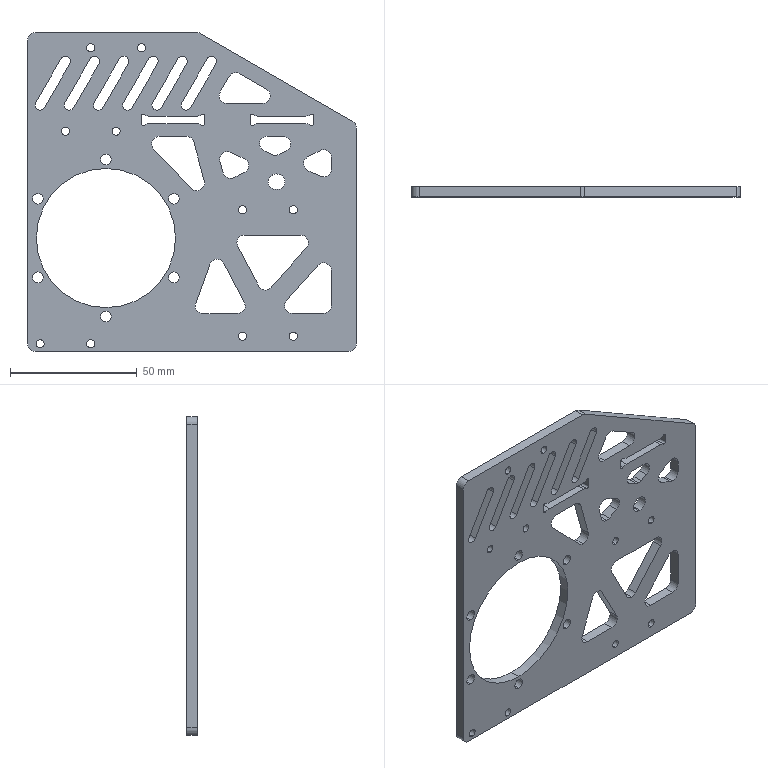Part | SolidWorks | features ICE 5, Fillet 2, Extrusion 1 | 1 solid | 163 faces | box 130 x 4 x 126 mm | volume 41493 mm3 | cylinder 109 | plane 54 | commonest cylinder face diameters 6 x45 3.2 x20 4 x18 1.5 x12 4.2 x12 55 x2